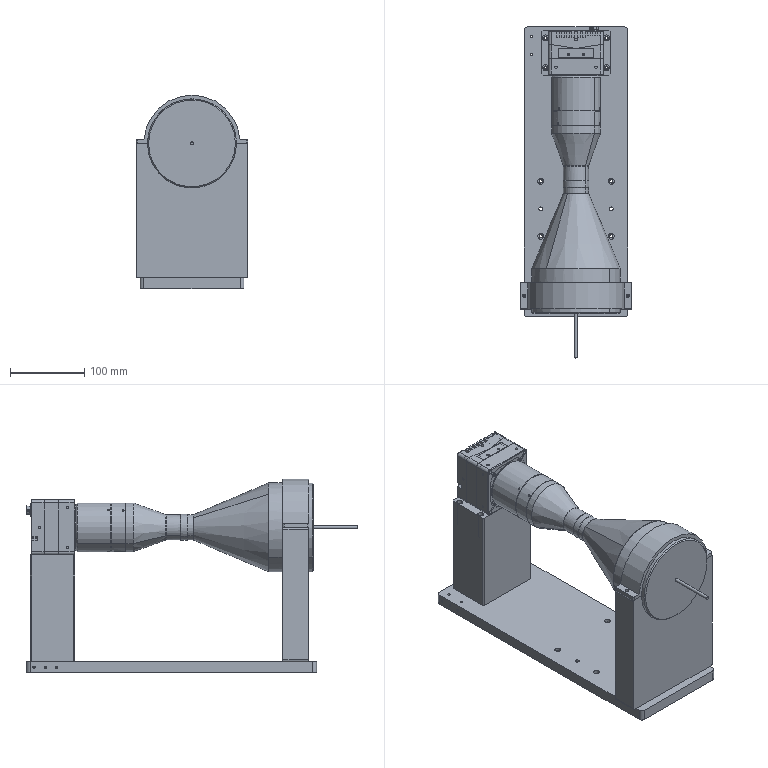Part | SolidWorks | features InContextFeatHolder 4, AEMSimFeature 1 | 29 solids | 2108 faces | box 150 x 447.19 x 260.95 mm | volume 4314882 mm3 | plane 1240 | cylinder 732 | cone 98 | spline 34 | torus 4 | commonest cylinder face diameters 2 x83 4.5 x67 3.3 x62 0.6 x56 8 x48 2.5 x44